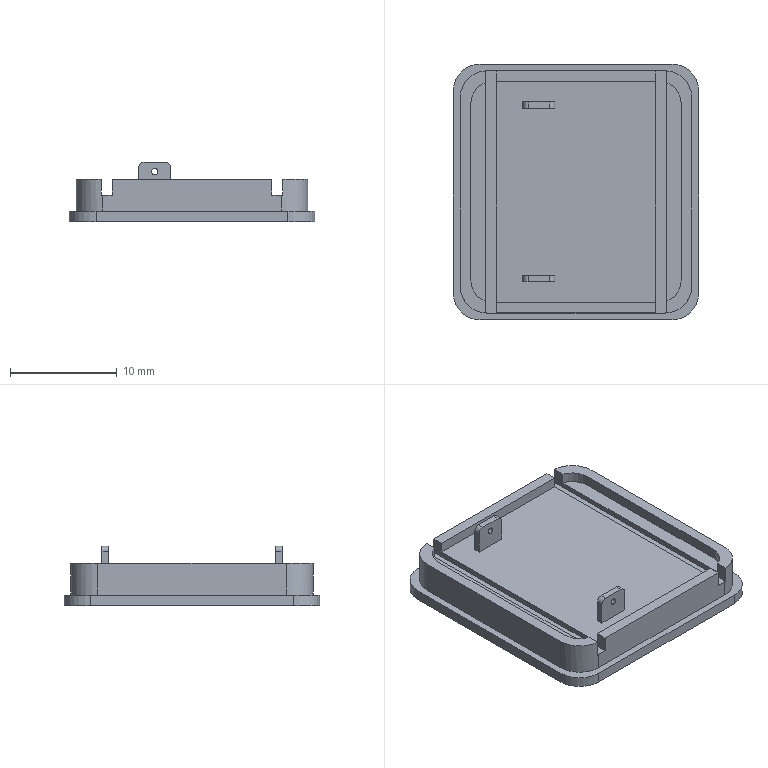Part | STEP file | product_Default | 1 solid | 57 faces | box 23 x 24 x 5.6 mm | volume 1586 mm3 | plane 37 | cylinder 20 | commonest cylinder face diameters 5 x8 0.6 x4 1 x4 4 x4